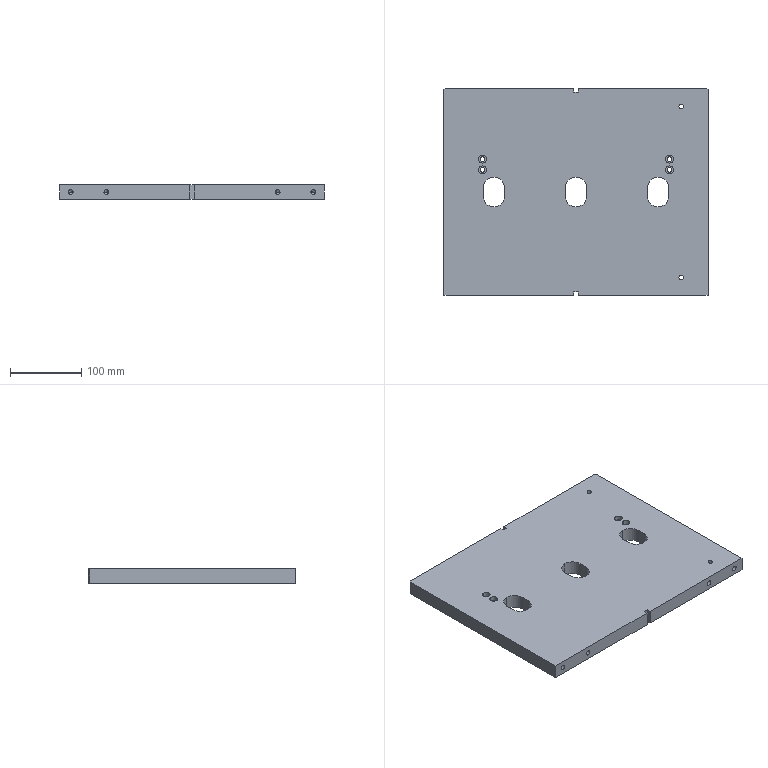Part | 1 solid | 93 faces | box 370 x 290 x 20 mm | volume 2068332 mm3 | cylinder 49 | plane 28 | cone 16 | commonest cylinder face diameters 6.8 x16 6.6 x12 11 x12 30 x9